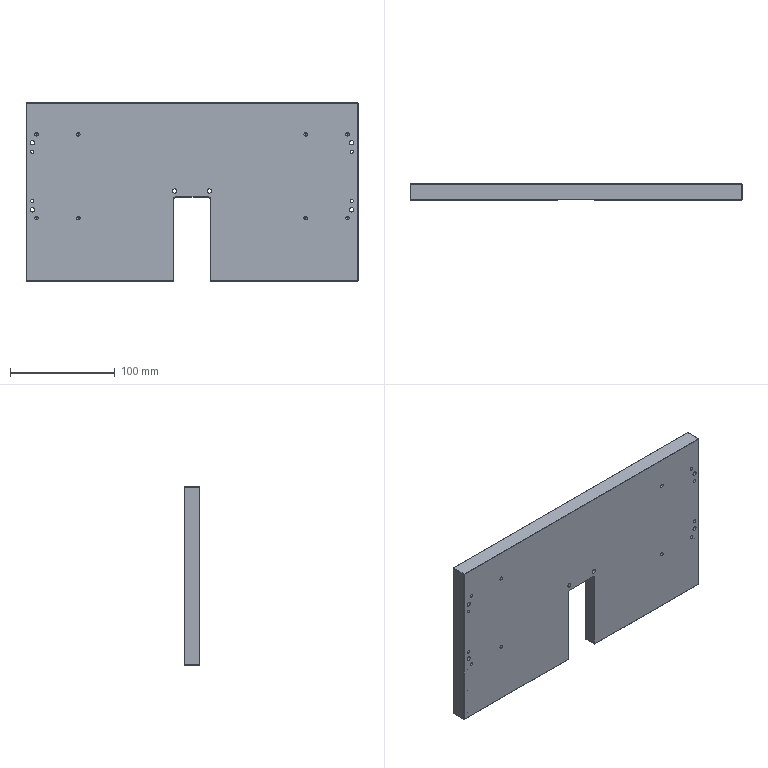Part | SolidWorks | features ICE 5, HoleWzd 4, Chamfer 2, Extrusion 1, Fillet 1 | 1 solid | 159 faces | box 317 x 15 x 170 mm | volume 619521 mm3 | cylinder 62 | plane 61 | cone 36 | commonest cylinder face diameters 3.3 x28 3 x12 4.2 x12 5 x8 4 x2